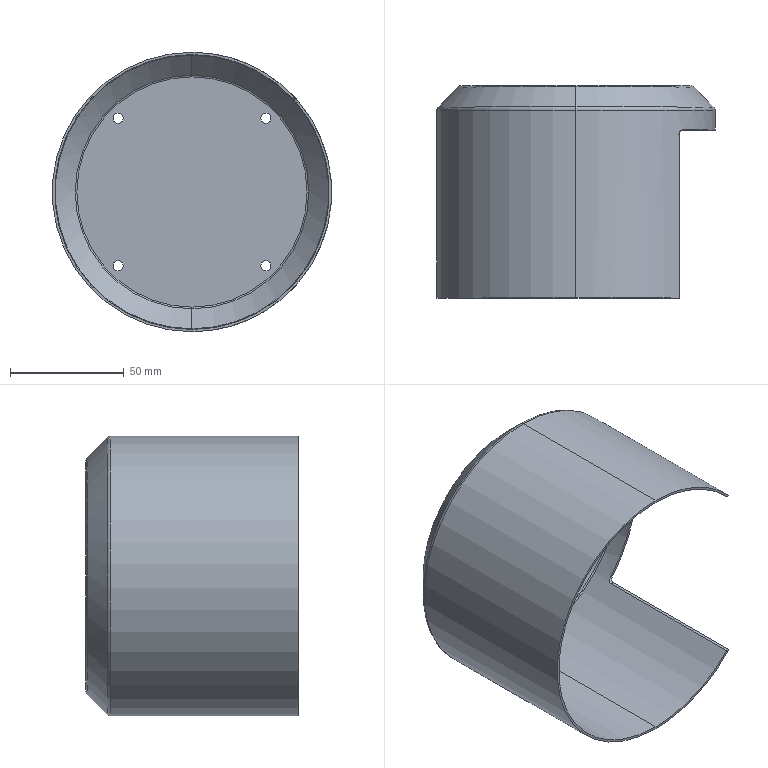Part | SolidWorks | features Fillet 2, Chamfer 1, Extrusion 1, HoleWzd 1, ICE 1, Shell 1 | 1 solid | 32 faces | box 123 x 93.5 x 123 mm | volume 38171 mm3 | cylinder 14 | torus 8 | plane 6 | cone 4 | commonest cylinder face diameters 4.5 x8 4 x2 121 x2 123 x2
STEP:
#1=CARTESIAN_POINT('',(-32.5,45.75,-34.75));
#2=VERTEX_POINT('',#1);
#3=CARTESIAN_POINT('',(-32.5,45.75,-30.25));
#4=VERTEX_POINT('',#3);
#5=CARTESIAN_POINT('',(-32.5,45.75,-32.5));
#6=DIRECTION('',(0.,1.,0.));
#7=DIRECTION('',(0.,0.,1.));
#8=AXIS2_PLACEMENT_3D('',#5,#6,#7);
#9=CIRCLE('',#8,2.25);
#10=EDGE_CURVE('',#2,#4,#9,.T.);
#11=ORIENTED_EDGE('',*,*,#10,.F.);
#12=CARTESIAN_POINT('',(-32.5,46.75,-34.75));
#13=VERTEX_POINT('',#12);
#14=CARTESIAN_POINT('',(-32.5,46.75,-34.75));
#15=DIRECTION('',(0.,1.,0.));
#16=VECTOR('',#15,1000.);
#17=LINE('',#14,#16);
#18=EDGE_CURVE('',#2,#13,#17,.T.);
#19=ORIENTED_EDGE('',*,*,#18,.T.);
#20=CARTESIAN_POINT('',(-32.5,46.75,-30.25));
#21=VERTEX_POINT('',#20);
#22=CARTESIAN_POINT('',(-32.5,46.75,-32.5));
#23=DIRECTION('',(0.,1.,0.));
#24=DIRECTION('',(0.,0.,1.));
#25=AXIS2_PLACEMENT_3D('',#22,#23,#24);
#26=CIRCLE('',#25,2.25);
#27=EDGE_CURVE('',#13,#21,#26,.T.);
#28=ORIENTED_EDGE('',*,*,#27,.T.);
#29=CARTESIAN_POINT('',(-32.5,46.75,-30.25));
#30=DIRECTION('',(0.,1.,0.));
#31=VECTOR('',#30,1000.);
#32=LINE('',#29,#31);
#33=EDGE_CURVE('',#4,#21,#32,.T.);
#34=ORIENTED_EDGE('',*,*,#33,.F.);
#35=EDGE_LOOP('',(#11,#19,#28,#34));
#36=FACE_OUTER_BOUND('',#35,.T.);
#37=CARTESIAN_POINT('',(-32.5,46.75,-32.5));
#38=DIRECTION('',(0.,1.,0.));
#39=DIRECTION('',(0.,0.,1.));
#40=AXIS2_PLACEMENT_3D('',#37,#38,#39);
#41=CYLINDRICAL_SURFACE('',#40,2.25);
#42=ADVANCED_FACE('',(#36),#41,.F.);
#43=CARTESIAN_POINT('',(32.5,45.75,-34.75));
#44=VERTEX_POINT('',#43);
#45=CARTESIAN_POINT('',(32.5,45.75,-30.25));
#46=VERTEX_POINT('',#45);
#47=CARTESIAN_POINT('',(32.5,45.75,-32.5));
#48=DIRECTION('',(0.,1.,0.));
#49=DIRECTION('',(0.,0.,1.));
#50=AXIS2_PLACEMENT_3D('',#47,#48,#49);
#51=CIRCLE('',#50,2.25);
#52=EDGE_CURVE('',#44,#46,#51,.T.);
#53=ORIENTED_EDGE('',*,*,#52,.F.);
#54=CARTESIAN_POINT('',(32.5,46.75,-34.75));
#55=VERTEX_POINT('',#54);
#56=CARTESIAN_POINT('',(32.5,46.75,-34.75));
#57=DIRECTION('',(0.,1.,0.));
#58=VECTOR('',#57,1000.);
#59=LINE('',#56,#58);
#60=EDGE_CURVE('',#44,#55,#59,.T.);
#61=ORIENTED_EDGE('',*,*,#60,.T.);
#62=CARTESIAN_POINT('',(32.5,46.75,-30.25));
#63=VERTEX_POINT('',#62);
#64=CARTESIAN_POINT('',(32.5,46.75,-32.5));
#65=DIRECTION('',(0.,1.,0.));
#66=DIRECTION('',(0.,0.,1.));
#67=AXIS2_PLACEMENT_3D('',#64,#65,#66);
#68=CIRCLE('',#67,2.25);
#69=EDGE_CURVE('',#55,#63,#68,.T.);
#70=ORIENTED_EDGE('',*,*,#69,.T.);
#71=CARTESIAN_POINT('',(32.5,46.75,-30.25));
#72=DIRECTION('',(0.,1.,0.));
#73=VECTOR('',#72,1000.);
#74=LINE('',#71,#73);
#75=EDGE_CURVE('',#46,#63,#74,.T.);
#76=ORIENTED_EDGE('',*,*,#75,.F.);
#77=EDGE_LOOP('',(#53,#61,#70,#76));
#78=FACE_OUTER_BOUND('',#77,.T.);
#79=CARTESIAN_POINT('',(32.5,46.75,-32.5));
#80=DIRECTION('',(0.,1.,0.));
#81=DIRECTION('',(0.,0.,1.));
#82=AXIS2_PLACEMENT_3D('',#79,#80,#81);
#83=CYLINDRICAL_SURFACE('',#82,2.25);
#84=ADVANCED_FACE('',(#78),#83,.F.);
#85=CARTESIAN_POINT('',(32.5,45.75,30.25));
#86=VERTEX_POINT('',#85);
#87=CARTESIAN_POINT('',(32.5,45.75,34.75));
#88=VERTEX_POINT('',#87);
#89=CARTESIAN_POINT('',(32.5,45.75,32.5));
#90=DIRECTION('',(0.,1.,0.));
#91=DIRECTION('',(0.,0.,1.));
#92=AXIS2_PLACEMENT_3D('',#89,#90,#91);
#93=CIRCLE('',#92,2.25);
#94=EDGE_CURVE('',#86,#88,#93,.T.);
#95=ORIENTED_EDGE('',*,*,#94,.F.);
#96=CARTESIAN_POINT('',(32.5,46.75,30.25));
#97=VERTEX_POINT('',#96);
#98=CARTESIAN_POINT('',(32.5,46.75,30.25));
#99=DIRECTION('',(0.,1.,0.));
#100=VECTOR('',#99,1000.);
#101=LINE('',#98,#100);
#102=EDGE_CURVE('',#86,#97,#101,.T.);
#103=ORIENTED_EDGE('',*,*,#102,.T.);
#104=CARTESIAN_POINT('',(32.5,46.75,34.75));
#105=VERTEX_POINT('',#104);
#106=CARTESIAN_POINT('',(32.5,46.75,32.5));
#107=DIRECTION('',(0.,1.,0.));
#108=DIRECTION('',(0.,0.,1.));
#109=AXIS2_PLACEMENT_3D('',#106,#107,#108);
#110=CIRCLE('',#109,2.25);
#111=EDGE_CURVE('',#97,#105,#110,.T.);
#112=ORIENTED_EDGE('',*,*,#111,.T.);
#113=CARTESIAN_POINT('',(32.5,46.75,34.75));
#114=DIRECTION('',(0.,1.,0.));
#115=VECTOR('',#114,1000.);
#116=LINE('',#113,#115);
#117=EDGE_CURVE('',#88,#105,#116,.T.);
#118=ORIENTED_EDGE('',*,*,#117,.F.);
#119=EDGE_LOOP('',(#95,#103,#112,#118));
#120=FACE_OUTER_BOUND('',#119,.T.);
#121=CARTESIAN_POINT('',(32.5,46.75,32.5));
#122=DIRECTION('',(0.,1.,0.));
#123=DIRECTION('',(0.,0.,1.));
#124=AXIS2_PLACEMENT_3D('',#121,#122,#123);
#125=CYLINDRICAL_SURFACE('',#124,2.25);
#126=ADVANCED_FACE('',(#120),#125,.F.);
#127=CARTESIAN_POINT('',(-32.5,45.75,30.25));
#128=VERTEX_POINT('',#127);
#129=CARTESIAN_POINT('',(-32.5,45.75,34.75));
#130=VERTEX_POINT('',#129);
#131=CARTESIAN_POINT('',(-32.5,45.75,32.5));
#132=DIRECTION('',(0.,1.,0.));
#133=DIRECTION('',(0.,0.,1.));
#134=AXIS2_PLACEMENT_3D('',#131,#132,#133);
#135=CIRCLE('',#134,2.25);
#136=EDGE_CURVE('',#128,#130,#135,.T.);
#137=ORIENTED_EDGE('',*,*,#136,.F.);
#138=CARTESIAN_POINT('',(-32.5,46.75,30.25));
#139=VERTEX_POINT('',#138);
#140=CARTESIAN_POINT('',(-32.5,46.75,30.25));
#141=DIRECTION('',(0.,1.,0.));
#142=VECTOR('',#141,1000.);
#143=LINE('',#140,#142);
#144=EDGE_CURVE('',#128,#139,#143,.T.);
#145=ORIENTED_EDGE('',*,*,#144,.T.);
#146=CARTESIAN_POINT('',(-32.5,46.75,34.75));
#147=VERTEX_POINT('',#146);
#148=CARTESIAN_POINT('',(-32.5,46.75,32.5));
#149=DIRECTION('',(0.,1.,0.));
#150=DIRECTION('',(0.,0.,1.));
#151=AXIS2_PLACEMENT_3D('',#148,#149,#150);
#152=CIRCLE('',#151,2.25);
#153=EDGE_CURVE('',#139,#147,#152,.T.);
#154=ORIENTED_EDGE('',*,*,#153,.T.);
#155=CARTESIAN_POINT('',(-32.5,46.75,34.75));
#156=DIRECTION('',(0.,1.,0.));
#157=VECTOR('',#156,1000.);
#158=LINE('',#155,#157);
#159=EDGE_CURVE('',#130,#147,#158,.T.);
#160=ORIENTED_EDGE('',*,*,#159,.F.);
#161=EDGE_LOOP('',(#137,#145,#154,#160));
#162=FACE_OUTER_BOUND('',#161,.T.);
#163=CARTESIAN_POINT('',(-32.5,46.75,32.5));
#164=DIRECTION('',(0.,1.,0.));
#165=DIRECTION('',(0.,0.,1.));
#166=AXIS2_PLACEMENT_3D('',#163,#164,#165);
#167=CYLINDRICAL_SURFACE('',#166,2.25);
#168=ADVANCED_FACE('',(#162),#167,.F.);
#169=CARTESIAN_POINT('',(0.,45.457,51.379));
#170=VERTEX_POINT('',#169);
#171=CARTESIAN_POINT('',(0.,45.457,-51.379));
#172=VERTEX_POINT('',#171);
#173=CARTESIAN_POINT('',(0.,45.457,0.));
#174=DIRECTION('',(0.,-1.,0.));
#175=DIRECTION('',(0.,0.,-1.));
#176=AXIS2_PLACEMENT_3D('',#173,#174,#175);
#177=CIRCLE('',#176,51.379);
#178=EDGE_CURVE('',#170,#172,#177,.T.);
#179=ORIENTED_EDGE('',*,*,#178,.T.);
#180=CARTESIAN_POINT('',(0.,45.75,-50.672));
#181=VERTEX_POINT('',#180);
#182=CARTESIAN_POINT('',(0.,44.75,-50.672));
#183=DIRECTION('',(1.,0.,0.));
#184=DIRECTION('',(0.,0.,-1.));
#185=AXIS2_PLACEMENT_3D('',#182,#183,#184);
#186=CIRCLE('',#185,1.);
#187=EDGE_CURVE('',#172,#181,#186,.T.);
#188=ORIENTED_EDGE('',*,*,#187,.T.);
#189=CARTESIAN_POINT('',(0.,45.75,50.672));
#190=VERTEX_POINT('',#189);
#191=CARTESIAN_POINT('',(0.,45.75,0.));
#192=DIRECTION('',(0.,1.,0.));
#193=DIRECTION('',(0.,0.,1.));
#194=AXIS2_PLACEMENT_3D('',#191,#192,#193);
#195=CIRCLE('',#194,50.672);
#196=EDGE_CURVE('',#181,#190,#195,.T.);
#197=ORIENTED_EDGE('',*,*,#196,.T.);
#198=CARTESIAN_POINT('',(0.,44.75,50.672));
#199=DIRECTION('',(-1.,0.,0.));
#200=DIRECTION('',(0.,0.,1.));
#201=AXIS2_PLACEMENT_3D('',#198,#199,#200);
#202=CIRCLE('',#201,1.);
#203=EDGE_CURVE('',#170,#190,#202,.T.);
#204=ORIENTED_EDGE('',*,*,#203,.F.);
#205=EDGE_LOOP('',(#179,#188,#197,#204));
#206=FACE_OUTER_BOUND('',#205,.T.);
#207=CARTESIAN_POINT('',(0.,44.75,0.));
#208=DIRECTION('',(0.,1.,0.));
#209=DIRECTION('',(0.,0.,1.));
#210=AXIS2_PLACEMENT_3D('',#207,#208,#209);
#211=TOROIDAL_SURFACE('',#210,50.672,1.);
#212=ADVANCED_FACE('',(#206),#211,.F.);
#213=CARTESIAN_POINT('',(0.,35.922,60.5));
#214=VERTEX_POINT('',#213);
#215=CARTESIAN_POINT('',(0.,35.922,-60.5));
#216=VERTEX_POINT('',#215);
#217=CARTESIAN_POINT('',(0.,35.922,0.));
#218=DIRECTION('',(0.,-1.,0.));
#219=DIRECTION('',(0.,0.,-1.));
#220=AXIS2_PLACEMENT_3D('',#217,#218,#219);
#221=CIRCLE('',#220,60.5);
#222=EDGE_CURVE('',#214,#216,#221,.T.);
#223=ORIENTED_EDGE('',*,*,#222,.T.);
#224=CARTESIAN_POINT('',(0.,36.629,-60.207));
#225=VERTEX_POINT('',#224);
#226=CARTESIAN_POINT('',(0.,35.922,-59.5));
#227=DIRECTION('',(1.,0.,0.));
#228=DIRECTION('',(0.,0.,-1.));
#229=AXIS2_PLACEMENT_3D('',#226,#227,#228);
#230=CIRCLE('',#229,1.);
#231=EDGE_CURVE('',#216,#225,#230,.T.);
#232=ORIENTED_EDGE('',*,*,#231,.T.);
#233=CARTESIAN_POINT('',(0.,36.629,60.207));
#234=VERTEX_POINT('',#233);
#235=CARTESIAN_POINT('',(0.,36.629,0.));
#236=DIRECTION('',(0.,1.,0.));
#237=DIRECTION('',(0.,0.,-1.));
#238=AXIS2_PLACEMENT_3D('',#235,#236,#237);
#239=CIRCLE('',#238,60.207);
#240=EDGE_CURVE('',#225,#234,#239,.T.);
#241=ORIENTED_EDGE('',*,*,#240,.T.);
#242=CARTESIAN_POINT('',(0.,35.922,59.5));
#243=DIRECTION('',(-1.,0.,0.));
#244=DIRECTION('',(0.,0.,1.));
#245=AXIS2_PLACEMENT_3D('',#242,#243,#244);
#246=CIRCLE('',#245,1.);
#247=EDGE_CURVE('',#214,#234,#246,.T.);
#248=ORIENTED_EDGE('',*,*,#247,.F.);
#249=EDGE_LOOP('',(#223,#232,#241,#248));
#250=FACE_OUTER_BOUND('',#249,.T.);
#251=CARTESIAN_POINT('',(0.,35.922,0.));
#252=DIRECTION('',(0.,1.,0.));
#253=DIRECTION('',(0.,0.,1.));
#254=AXIS2_PLACEMENT_3D('',#251,#252,#253);
#255=TOROIDAL_SURFACE('',#254,59.5,1.);
#256=ADVANCED_FACE('',(#250),#255,.F.);
#257=ORIENTED_EDGE('',*,*,#178,.F.);
#258=CARTESIAN_POINT('',(0.,46.043,50.793));
#259=DIRECTION('',(0.,-0.7071,0.7071));
#260=VECTOR('',#259,1000.);
#261=LINE('',#258,#260);
#262=EDGE_CURVE('',#170,#234,#261,.T.);
#263=ORIENTED_EDGE('',*,*,#262,.T.);
#264=ORIENTED_EDGE('',*,*,#240,.F.);
#265=CARTESIAN_POINT('',(0.,46.043,-50.793));
#266=DIRECTION('',(0.,-0.7071,-0.7071));
#267=VECTOR('',#266,1000.);
#268=LINE('',#265,#267);
#269=EDGE_CURVE('',#172,#225,#268,.T.);
#270=ORIENTED_EDGE('',*,*,#269,.F.);
#271=EDGE_LOOP('',(#257,#263,#264,#270));
#272=FACE_OUTER_BOUND('',#271,.T.);
#273=CARTESIAN_POINT('',(0.,46.043,0.));
#274=DIRECTION('',(0.,-1.,0.));
#275=DIRECTION('',(0.,0.,-1.));
#276=AXIS2_PLACEMENT_3D('',#273,#274,#275);
#277=CONICAL_SURFACE('',#276,50.793,0.7854);
#278=ADVANCED_FACE('',(#272),#277,.F.);
#279=ORIENTED_EDGE('',*,*,#222,.F.);
#280=CARTESIAN_POINT('',(0.,-46.75,60.5));
#281=VERTEX_POINT('',#280);
#282=CARTESIAN_POINT('',(0.,46.75,60.5));
#283=DIRECTION('',(0.,-1.,0.));
#284=VECTOR('',#283,1000.);
#285=LINE('',#282,#284);
#286=EDGE_CURVE('',#214,#281,#285,.T.);
#287=ORIENTED_EDGE('',*,*,#286,.T.);
#288=CARTESIAN_POINT('',(0.,-46.75,-60.5));
#289=VERTEX_POINT('',#288);
#290=CARTESIAN_POINT('',(0.,-46.75,0.));
#291=DIRECTION('',(0.,1.,0.));
#292=DIRECTION('',(0.,0.,1.));
#293=AXIS2_PLACEMENT_3D('',#290,#291,#292);
#294=CIRCLE('',#293,60.5);
#295=EDGE_CURVE('',#289,#281,#294,.T.);
#296=ORIENTED_EDGE('',*,*,#295,.F.);
#297=CARTESIAN_POINT('',(0.,46.75,-60.5));
#298=DIRECTION('',(0.,-1.,0.));
#299=VECTOR('',#298,1000.);
#300=LINE('',#297,#299);
#301=EDGE_CURVE('',#216,#289,#300,.T.);
#302=ORIENTED_EDGE('',*,*,#301,.F.);
#303=EDGE_LOOP('',(#279,#287,#296,#302));
#304=FACE_OUTER_BOUND('',#303,.T.);
#305=CARTESIAN_POINT('',(0.,46.75,0.));
#306=DIRECTION('',(0.,-1.,0.));
#307=DIRECTION('',(0.,0.,-1.));
#308=AXIS2_PLACEMENT_3D('',#305,#306,#307);
#309=CYLINDRICAL_SURFACE('',#308,60.5);
#310=ADVANCED_FACE('',(#304),#309,.F.);
#311=CARTESIAN_POINT('',(0.,46.164,-52.086));
#312=VERTEX_POINT('',#311);
#313=CARTESIAN_POINT('',(0.,46.164,52.086));
#314=VERTEX_POINT('',#313);
#315=CARTESIAN_POINT('',(0.,46.164,0.));
#316=DIRECTION('',(0.,-1.,0.));
#317=DIRECTION('',(0.,0.,1.));
#318=AXIS2_PLACEMENT_3D('',#315,#316,#317);
#319=CIRCLE('',#318,52.086);
#320=EDGE_CURVE('',#312,#314,#319,.T.);
#321=ORIENTED_EDGE('',*,*,#320,.F.);
#322=CARTESIAN_POINT('',(0.,46.75,-50.672));
#323=VERTEX_POINT('',#322);
#324=CARTESIAN_POINT('',(0.,44.75,-50.672));
#325=DIRECTION('',(1.,0.,0.));
#326=DIRECTION('',(0.,0.,-1.));
#327=AXIS2_PLACEMENT_3D('',#324,#325,#326);
#328=CIRCLE('',#327,2.);
#329=EDGE_CURVE('',#312,#323,#328,.T.);
#330=ORIENTED_EDGE('',*,*,#329,.T.);
#331=CARTESIAN_POINT('',(0.,46.75,50.672));
#332=VERTEX_POINT('',#331);
#333=CARTESIAN_POINT('',(0.,46.75,0.));
#334=DIRECTION('',(0.,1.,0.));
#335=DIRECTION('',(0.,0.,1.));
#336=AXIS2_PLACEMENT_3D('',#333,#334,#335);
#337=CIRCLE('',#336,50.672);
#338=EDGE_CURVE('',#332,#323,#337,.T.);
#339=ORIENTED_EDGE('',*,*,#338,.F.);
#340=CARTESIAN_POINT('',(0.,44.75,50.672));
#341=DIRECTION('',(-1.,0.,0.));
#342=DIRECTION('',(0.,0.,1.));
#343=AXIS2_PLACEMENT_3D('',#340,#341,#342);
#344=CIRCLE('',#343,2.);
#345=EDGE_CURVE('',#314,#332,#344,.T.);
#346=ORIENTED_EDGE('',*,*,#345,.F.);
#347=EDGE_LOOP('',(#321,#330,#339,#346));
#348=FACE_OUTER_BOUND('',#347,.T.);
#349=CARTESIAN_POINT('',(0.,44.75,0.));
#350=DIRECTION('',(0.,1.,0.));
#351=DIRECTION('',(0.,0.,1.));
#352=AXIS2_PLACEMENT_3D('',#349,#350,#351);
#353=TOROIDAL_SURFACE('',#352,50.672,2.);
#354=ADVANCED_FACE('',(#348),#353,.T.);
#355=CARTESIAN_POINT('',(0.,35.922,-61.5));
#356=VERTEX_POINT('',#355);
#357=CARTESIAN_POINT('',(0.,35.922,61.5));
#358=VERTEX_POINT('',#357);
#359=CARTESIAN_POINT('',(0.,35.922,0.));
#360=DIRECTION('',(0.,-1.,0.));
#361=DIRECTION('',(0.,0.,1.));
#362=AXIS2_PLACEMENT_3D('',#359,#360,#361);
#363=CIRCLE('',#362,61.5);
#364=EDGE_CURVE('',#356,#358,#363,.T.);
#365=ORIENTED_EDGE('',*,*,#364,.F.);
#366=CARTESIAN_POINT('',(0.,37.336,-60.914));
#367=VERTEX_POINT('',#366);
#368=CARTESIAN_POINT('',(0.,35.922,-59.5));
#369=DIRECTION('',(1.,0.,0.));
#370=DIRECTION('',(0.,0.,-1.));
#371=AXIS2_PLACEMENT_3D('',#368,#369,#370);
#372=CIRCLE('',#371,2.);
#373=EDGE_CURVE('',#356,#367,#372,.T.);
#374=ORIENTED_EDGE('',*,*,#373,.T.);
#375=CARTESIAN_POINT('',(0.,37.336,60.914));
#376=VERTEX_POINT('',#375);
#377=CARTESIAN_POINT('',(0.,37.336,0.));
#378=DIRECTION('',(0.,1.,0.));
#379=DIRECTION('',(0.,0.,-1.));
#380=AXIS2_PLACEMENT_3D('',#377,#378,#379);
#381=CIRCLE('',#380,60.914);
#382=EDGE_CURVE('',#376,#367,#381,.T.);
#383=ORIENTED_EDGE('',*,*,#382,.F.);
#384=CARTESIAN_POINT('',(0.,35.922,59.5));
#385=DIRECTION('',(-1.,0.,0.));
#386=DIRECTION('',(0.,0.,1.));
#387=AXIS2_PLACEMENT_3D('',#384,#385,#386);
#388=CIRCLE('',#387,2.);
#389=EDGE_CURVE('',#358,#376,#388,.T.);
#390=ORIENTED_EDGE('',*,*,#389,.F.);
#391=EDGE_LOOP('',(#365,#374,#383,#390));
#392=FACE_OUTER_BOUND('',#391,.T.);
#393=CARTESIAN_POINT('',(0.,35.922,0.));
#394=DIRECTION('',(0.,1.,0.));
#395=DIRECTION('',(0.,0.,1.));
#396=AXIS2_PLACEMENT_3D('',#393,#394,#395);
#397=TOROIDAL_SURFACE('',#396,59.5,2.);
#398=ADVANCED_FACE('',(#392),#397,.T.);
#399=ORIENTED_EDGE('',*,*,#320,.T.);
#400=CARTESIAN_POINT('',(0.,46.75,51.5));
#401=DIRECTION('',(0.,-0.7071,0.7071));
#402=VECTOR('',#401,1000.);
#403=LINE('',#400,#402);
#404=EDGE_CURVE('',#314,#376,#403,.T.);
#405=ORIENTED_EDGE('',*,*,#404,.T.);
#406=ORIENTED_EDGE('',*,*,#382,.T.);
#407=CARTESIAN_POINT('',(0.,46.75,-51.5));
#408=DIRECTION('',(0.,-0.7071,-0.7071));
#409=VECTOR('',#408,1000.);
#410=LINE('',#407,#409);
#411=EDGE_CURVE('',#312,#367,#410,.T.);
#412=ORIENTED_EDGE('',*,*,#411,.F.);
#413=EDGE_LOOP('',(#399,#405,#406,#412));
#414=FACE_OUTER_BOUND('',#413,.T.);
#415=CARTESIAN_POINT('',(0.,46.75,0.));
#416=DIRECTION('',(0.,-1.,0.));
#417=DIRECTION('',(0.,0.,-1.));
#418=AXIS2_PLACEMENT_3D('',#415,#416,#417);
#419=CONICAL_SURFACE('',#418,51.5,0.7854);
#420=ADVANCED_FACE('',(#414),#419,.T.);
#421=ORIENTED_EDGE('',*,*,#364,.T.);
#422=CARTESIAN_POINT('',(0.,-46.75,61.5));
#423=VERTEX_POINT('',#422);
#424=CARTESIAN_POINT('',(0.,46.75,61.5));
#425=DIRECTION('',(0.,-1.,0.));
#426=VECTOR('',#425,1000.);
#427=LINE('',#424,#426);
#428=EDGE_CURVE('',#358,#423,#427,.T.);
#429=ORIENTED_EDGE('',*,*,#428,.T.);
#430=CARTESIAN_POINT('',(45.387,-46.75,41.5));
#431=VERTEX_POINT('',#430);
#432=CARTESIAN_POINT('',(0.,-46.75,0.));
#433=DIRECTION('',(0.,1.,0.));
#434=DIRECTION('',(0.,0.,1.));
#435=AXIS2_PLACEMENT_3D('',#432,#433,#434);
#436=CIRCLE('',#435,61.5);
#437=EDGE_CURVE('',#423,#431,#436,.T.);
#438=ORIENTED_EDGE('',*,*,#437,.T.);
#439=CARTESIAN_POINT('',(45.387,25.25,41.5));
#440=VERTEX_POINT('',#439);
#441=CARTESIAN_POINT('',(45.387,46.75,41.5));
#442=DIRECTION('',(0.,1.,0.));
#443=VECTOR('',#442,1000.);
#444=LINE('',#441,#443);
#445=EDGE_CURVE('',#431,#440,#444,.T.);
#446=ORIENTED_EDGE('',*,*,#445,.T.);
#447=CARTESIAN_POINT('',(47.138,27.25,39.5));
#448=VERTEX_POINT('',#447);
#449=CARTESIAN_POINT('',(45.387,25.25,41.5));
#450=CARTESIAN_POINT('',(45.387,25.405,41.5));
#451=CARTESIAN_POINT('',(45.403,25.555,41.482));
#452=CARTESIAN_POINT('',(45.465,25.848,41.414));
#453=CARTESIAN_POINT('',(45.511,25.988,41.364));
#454=CARTESIAN_POINT('',(45.623,26.245,41.241));
#455=CARTESIAN_POINT('',(45.69,26.364,41.166));
#456=CARTESIAN_POINT('',(45.837,26.576,41.003));
#457=CARTESIAN_POINT('',(45.916,26.67,40.914));
#458=CARTESIAN_POINT('',(46.173,26.923,40.625));
#459=CARTESIAN_POINT('',(46.357,27.044,40.415));
#460=CARTESIAN_POINT('',(46.743,27.209,39.968));
#461=CARTESIAN_POINT('',(46.941,27.25,39.736));
#462=CARTESIAN_POINT('',(47.138,27.25,39.5));
#463=B_SPLINE_CURVE_WITH_KNOTS('',3,(#449,#450,#451,#452,#453,#454,#455,#456,#457,#458,#459,#460,#461,#462),.UNSPECIFIED.,.F.,.F.,(4,2,2,2,2,2,4),(0.,0.0004571,0.0009142,0.001371,0.001828,0.002743,0.003657),.UNSPECIFIED.);
#464=EDGE_CURVE('',#440,#448,#463,.T.);
#465=ORIENTED_EDGE('',*,*,#464,.T.);
#466=CARTESIAN_POINT('',(47.138,27.25,-39.5));
#467=VERTEX_POINT('',#466);
#468=CARTESIAN_POINT('',(0.,27.25,0.));
#469=DIRECTION('',(0.,-1.,0.));
#470=DIRECTION('',(0.,0.,-1.));
#471=AXIS2_PLACEMENT_3D('',#468,#469,#470);
#472=CIRCLE('',#471,61.5);
#473=EDGE_CURVE('',#467,#448,#472,.T.);
#474=ORIENTED_EDGE('',*,*,#473,.F.);
#475=CARTESIAN_POINT('',(45.387,25.25,-41.5));
#476=VERTEX_POINT('',#475);
#477=CARTESIAN_POINT('',(47.138,27.25,-39.5));
#478=CARTESIAN_POINT('',(46.94,27.25,-39.736));
#479=CARTESIAN_POINT('',(46.745,27.21,-39.965));
#480=CARTESIAN_POINT('',(46.359,27.046,-40.413));
#481=CARTESIAN_POINT('',(46.173,26.924,-40.624));
#482=CARTESIAN_POINT('',(45.833,26.589,-41.008));
#483=CARTESIAN_POINT('',(45.68,26.375,-41.178));
#484=CARTESIAN_POINT('',(45.511,25.989,-41.364));
#485=CARTESIAN_POINT('',(45.466,25.852,-41.413));
#486=CARTESIAN_POINT('',(45.404,25.557,-41.482));
#487=CARTESIAN_POINT('',(45.387,25.405,-41.5));
#488=CARTESIAN_POINT('',(45.387,25.25,-41.5));
#489=B_SPLINE_CURVE_WITH_KNOTS('',3,(#477,#478,#479,#480,#481,#482,#483,#484,#485,#486,#487,#488),.UNSPECIFIED.,.F.,.F.,(4,2,2,2,2,4),(0.,0.0009127,0.001825,0.002738,0.003194,0.003651),.UNSPECIFIED.);
#490=EDGE_CURVE('',#467,#476,#489,.T.);
#491=ORIENTED_EDGE('',*,*,#490,.T.);
#492=CARTESIAN_POINT('',(45.387,-46.75,-41.5));
#493=VERTEX_POINT('',#492);
#494=CARTESIAN_POINT('',(45.387,46.75,-41.5));
#495=DIRECTION('',(0.,-1.,0.));
#496=VECTOR('',#495,1000.);
#497=LINE('',#494,#496);
#498=EDGE_CURVE('',#476,#493,#497,.T.);
#499=ORIENTED_EDGE('',*,*,#498,.T.);
#500=CARTESIAN_POINT('',(0.,-46.75,-61.5));
#501=VERTEX_POINT('',#500);
#502=CARTESIAN_POINT('',(0.,-46.75,0.));
#503=DIRECTION('',(0.,1.,0.));
#504=DIRECTION('',(0.,0.,1.));
#505=AXIS2_PLACEMENT_3D('',#502,#503,#504);
#506=CIRCLE('',#505,61.5);
#507=EDGE_CURVE('',#493,#501,#506,.T.);
#508=ORIENTED_EDGE('',*,*,#507,.T.);
#509=CARTESIAN_POINT('',(0.,46.75,-61.5));
#510=DIRECTION('',(0.,-1.,0.));
#511=VECTOR('',#510,1000.);
#512=LINE('',#509,#511);
#513=EDGE_CURVE('',#356,#501,#512,.T.);
#514=ORIENTED_EDGE('',*,*,#513,.F.);
#515=EDGE_LOOP('',(#421,#429,#438,#446,#465,#474,#491,#499,#508,#514));
#516=FACE_OUTER_BOUND('',#515,.T.);
#517=CARTESIAN_POINT('',(0.,46.75,0.));
#518=DIRECTION('',(0.,-1.,0.));
#519=DIRECTION('',(0.,0.,-1.));
#520=AXIS2_PLACEMENT_3D('',#517,#518,#519);
#521=CYLINDRICAL_SURFACE('',#520,61.5);
#522=ADVANCED_FACE('',(#516),#521,.T.);
#523=ORIENTED_EDGE('',*,*,#428,.F.);
#524=CARTESIAN_POINT('',(0.,35.922,0.));
#525=DIRECTION('',(0.,-1.,0.));
#526=DIRECTION('',(0.,0.,1.));
#527=AXIS2_PLACEMENT_3D('',#524,#525,#526);
#528=CIRCLE('',#527,61.5);
#529=EDGE_CURVE('',#358,#356,#528,.T.);
#530=ORIENTED_EDGE('',*,*,#529,.T.);
#531=ORIENTED_EDGE('',*,*,#513,.T.);
#532=CARTESIAN_POINT('',(0.,-46.75,0.));
#533=DIRECTION('',(0.,1.,0.));
#534=DIRECTION('',(0.,0.,1.));
#535=AXIS2_PLACEMENT_3D('',#532,#533,#534);
#536=CIRCLE('',#535,61.5);
#537=EDGE_CURVE('',#501,#423,#536,.T.);
#538=ORIENTED_EDGE('',*,*,#537,.T.);
#539=EDGE_LOOP('',(#523,#530,#531,#538));
#540=FACE_OUTER_BOUND('',#539,.T.);
#541=CARTESIAN_POINT('',(0.,46.75,0.));
#542=DIRECTION('',(0.,-1.,0.));
#543=DIRECTION('',(0.,0.,-1.));
#544=AXIS2_PLACEMENT_3D('',#541,#542,#543);
#545=CYLINDRICAL_SURFACE('',#544,61.5);
#546=ADVANCED_FACE('',(#540),#545,.T.);
#547=CARTESIAN_POINT('',(-32.5,46.75,-32.5));
#548=DIRECTION('',(0.,1.,0.));
#549=DIRECTION('',(0.,0.,1.));
#550=AXIS2_PLACEMENT_3D('',#547,#548,#549);
#551=CIRCLE('',#550,2.25);
#552=EDGE_CURVE('',#21,#13,#551,.T.);
#553=ORIENTED_EDGE('',*,*,#552,.F.);
#554=ORIENTED_EDGE('',*,*,#27,.F.);
#555=EDGE_LOOP('',(#553,#554));
#556=FACE_BOUND('',#555,.T.);
#557=CARTESIAN_POINT('',(32.5,46.75,-32.5));
#558=DIRECTION('',(0.,1.,0.));
#559=DIRECTION('',(0.,0.,1.));
#560=AXIS2_PLACEMENT_3D('',#557,#558,#559);
#561=CIRCLE('',#560,2.25);
#562=EDGE_CURVE('',#63,#55,#561,.T.);
#563=ORIENTED_EDGE('',*,*,#562,.F.);
#564=ORIENTED_EDGE('',*,*,#69,.F.);
#565=EDGE_LOOP('',(#563,#564));
#566=FACE_BOUND('',#565,.T.);
#567=CARTESIAN_POINT('',(32.5,46.75,32.5));
#568=DIRECTION('',(0.,1.,0.));
#569=DIRECTION('',(0.,0.,1.));
#570=AXIS2_PLACEMENT_3D('',#567,#568,#569);
#571=CIRCLE('',#570,2.25);
#572=EDGE_CURVE('',#105,#97,#571,.T.);
#573=ORIENTED_EDGE('',*,*,#572,.F.);
#574=ORIENTED_EDGE('',*,*,#111,.F.);
#575=EDGE_LOOP('',(#573,#574));
#576=FACE_BOUND('',#575,.T.);
#577=CARTESIAN_POINT('',(-32.5,46.75,32.5));
#578=DIRECTION('',(0.,1.,0.));
#579=DIRECTION('',(0.,0.,1.));
#580=AXIS2_PLACEMENT_3D('',#577,#578,#579);
#581=CIRCLE('',#580,2.25);
#582=EDGE_CURVE('',#147,#139,#581,.T.);
#583=ORIENTED_EDGE('',*,*,#582,.F.);
#584=ORIENTED_EDGE('',*,*,#153,.F.);
#585=EDGE_LOOP('',(#583,#584));
#586=FACE_BOUND('',#585,.T.);
#587=ORIENTED_EDGE('',*,*,#338,.T.);
#588=CARTESIAN_POINT('',(0.,46.75,0.));
#589=DIRECTION('',(0.,1.,0.));
#590=DIRECTION('',(0.,0.,1.));
#591=AXIS2_PLACEMENT_3D('',#588,#589,#590);
#592=CIRCLE('',#591,50.672);
#593=EDGE_CURVE('',#323,#332,#592,.T.);
#594=ORIENTED_EDGE('',*,*,#593,.T.);
#595=EDGE_LOOP('',(#587,#594));
#596=FACE_OUTER_BOUND('',#595,.T.);
#597=CARTESIAN_POINT('',(0.,46.75,0.));
#598=DIRECTION('',(0.,1.,0.));
#599=DIRECTION('',(0.,0.,1.));
#600=AXIS2_PLACEMENT_3D('',#597,#598,#599);
#601=PLANE('',#600);
#602=ADVANCED_FACE('',(#556,#566,#576,#586,#596),#601,.T.);
#603=ORIENTED_EDGE('',*,*,#507,.F.);
#604=CARTESIAN_POINT('',(44.023,-46.75,-41.5));
#605=VERTEX_POINT('',#604);
#606=CARTESIAN_POINT('',(-5.,-46.75,-41.5));
#607=DIRECTION('',(1.,0.,0.));
#608=VECTOR('',#607,1000.);
#609=LINE('',#606,#608);
#610=EDGE_CURVE('',#605,#493,#609,.T.);
#611=ORIENTED_EDGE('',*,*,#610,.F.);
#612=CARTESIAN_POINT('',(0.,-46.75,0.));
#613=DIRECTION('',(0.,1.,0.));
#614=DIRECTION('',(0.,0.,1.));
#615=AXIS2_PLACEMENT_3D('',#612,#613,#614);
#616=CIRCLE('',#615,60.5);
#617=EDGE_CURVE('',#605,#289,#616,.T.);
#618=ORIENTED_EDGE('',*,*,#617,.T.);
#619=ORIENTED_EDGE('',*,*,#295,.T.);
#620=CARTESIAN_POINT('',(44.023,-46.75,41.5));
#621=VERTEX_POINT('',#620);
#622=CARTESIAN_POINT('',(0.,-46.75,0.));
#623=DIRECTION('',(0.,1.,0.));
#624=DIRECTION('',(0.,0.,1.));
#625=AXIS2_PLACEMENT_3D('',#622,#623,#624);
#626=CIRCLE('',#625,60.5);
#627=EDGE_CURVE('',#281,#621,#626,.T.);
#628=ORIENTED_EDGE('',*,*,#627,.T.);
#629=CARTESIAN_POINT('',(-5.,-46.75,41.5));
#630=DIRECTION('',(-1.,0.,0.));
#631=VECTOR('',#630,1000.);
#632=LINE('',#629,#631);
#633=EDGE_CURVE('',#431,#621,#632,.T.);
#634=ORIENTED_EDGE('',*,*,#633,.F.);
#635=ORIENTED_EDGE('',*,*,#437,.F.);
#636=ORIENTED_EDGE('',*,*,#537,.F.);
#637=EDGE_LOOP('',(#603,#611,#618,#619,#628,#634,#635,#636));
#638=FACE_OUTER_BOUND('',#637,.T.);
#639=CARTESIAN_POINT('',(0.,-46.75,0.));
#640=DIRECTION('',(0.,1.,0.));
#641=DIRECTION('',(0.,0.,1.));
#642=AXIS2_PLACEMENT_3D('',#639,#640,#641);
#643=PLANE('',#642);
#644=ADVANCED_FACE('',(#638),#643,.F.);
#645=ORIENTED_EDGE('',*,*,#404,.F.);
#646=CARTESIAN_POINT('',(0.,46.164,0.));
#647=DIRECTION('',(0.,-1.,0.));
#648=DIRECTION('',(0.,0.,1.));
#649=AXIS2_PLACEMENT_3D('',#646,#647,#648);
#650=CIRCLE('',#649,52.086);
#651=EDGE_CURVE('',#314,#312,#650,.T.);
#652=ORIENTED_EDGE('',*,*,#651,.T.);
#653=ORIENTED_EDGE('',*,*,#411,.T.);
#654=CARTESIAN_POINT('',(0.,37.336,0.));
#655=DIRECTION('',(0.,1.,0.));
#656=DIRECTION('',(0.,0.,-1.));
#657=AXIS2_PLACEMENT_3D('',#654,#655,#656);
#658=CIRCLE('',#657,60.914);
#659=EDGE_CURVE('',#367,#376,#658,.T.);
#660=ORIENTED_EDGE('',*,*,#659,.T.);
#661=EDGE_LOOP('',(#645,#652,#653,#660));
#662=FACE_OUTER_BOUND('',#661,.T.);
#663=CARTESIAN_POINT('',(0.,46.75,0.));
#664=DIRECTION('',(0.,-1.,0.));
#665=DIRECTION('',(0.,0.,-1.));
#666=AXIS2_PLACEMENT_3D('',#663,#664,#665);
#667=CONICAL_SURFACE('',#666,51.5,0.7854);
#668=ADVANCED_FACE('',(#662),#667,.T.);
#669=ORIENTED_EDGE('',*,*,#373,.F.);
#670=ORIENTED_EDGE('',*,*,#529,.F.);
#671=ORIENTED_EDGE('',*,*,#389,.T.);
#672=ORIENTED_EDGE('',*,*,#659,.F.);
#673=EDGE_LOOP('',(#669,#670,#671,#672));
#674=FACE_OUTER_BOUND('',#673,.T.);
#675=CARTESIAN_POINT('',(0.,35.922,0.));
#676=DIRECTION('',(0.,1.,0.));
#677=DIRECTION('',(0.,0.,1.));
#678=AXIS2_PLACEMENT_3D('',#675,#676,#677);
#679=TOROIDAL_SURFACE('',#678,59.5,2.);
#680=ADVANCED_FACE('',(#674),#679,.T.);
#681=ORIENTED_EDGE('',*,*,#329,.F.);
#682=ORIENTED_EDGE('',*,*,#651,.F.);
#683=ORIENTED_EDGE('',*,*,#345,.T.);
#684=ORIENTED_EDGE('',*,*,#593,.F.);
#685=EDGE_LOOP('',(#681,#682,#683,#684));
#686=FACE_OUTER_BOUND('',#685,.T.);
#687=CARTESIAN_POINT('',(0.,44.75,0.));
#688=DIRECTION('',(0.,1.,0.));
#689=DIRECTION('',(0.,0.,1.));
#690=AXIS2_PLACEMENT_3D('',#687,#688,#689);
#691=TOROIDAL_SURFACE('',#690,50.672,2.);
#692=ADVANCED_FACE('',(#686),#691,.T.);
#693=ORIENTED_EDGE('',*,*,#286,.F.);
#694=CARTESIAN_POINT('',(0.,35.922,0.));
#695=DIRECTION('',(0.,-1.,0.));
#696=DIRECTION('',(0.,0.,-1.));
#697=AXIS2_PLACEMENT_3D('',#694,#695,#696);
#698=CIRCLE('',#697,60.5);
#699=EDGE_CURVE('',#216,#214,#698,.T.);
#700=ORIENTED_EDGE('',*,*,#699,.F.);
#701=ORIENTED_EDGE('',*,*,#301,.T.);
#702=ORIENTED_EDGE('',*,*,#617,.F.);
#703=CARTESIAN_POINT('',(44.023,25.25,-41.5));
#704=VERTEX_POINT('',#703);
#705=CARTESIAN_POINT('',(44.023,46.75,-41.5));
#706=DIRECTION('',(0.,-1.,0.));
#707=VECTOR('',#706,1000.);
#708=LINE('',#705,#707);
#709=EDGE_CURVE('',#704,#605,#708,.T.);
#710=ORIENTED_EDGE('',*,*,#709,.F.);
#711=CARTESIAN_POINT('',(45.826,27.25,-39.5));
#712=VERTEX_POINT('',#711);
#713=CARTESIAN_POINT('',(44.023,25.25,-41.5));
#714=CARTESIAN_POINT('',(44.023,25.406,-41.5));
#715=CARTESIAN_POINT('',(44.04,25.558,-41.482));
#716=CARTESIAN_POINT('',(44.105,25.853,-41.413));
#717=CARTESIAN_POINT('',(44.152,25.993,-41.362));
#718=CARTESIAN_POINT('',(44.268,26.25,-41.238));
#719=CARTESIAN_POINT('',(44.338,26.369,-41.163));
#720=CARTESIAN_POINT('',(44.49,26.58,-40.999));
#721=CARTESIAN_POINT('',(44.572,26.674,-40.91));
#722=CARTESIAN_POINT('',(44.836,26.926,-40.62));
#723=CARTESIAN_POINT('',(45.025,27.046,-40.411));
#724=CARTESIAN_POINT('',(45.421,27.209,-39.966));
#725=CARTESIAN_POINT('',(45.623,27.25,-39.735));
#726=CARTESIAN_POINT('',(45.826,27.25,-39.5));
#727=B_SPLINE_CURVE_WITH_KNOTS('',3,(#713,#714,#715,#716,#717,#718,#719,#720,#721,#722,#723,#724,#725,#726),.UNSPECIFIED.,.F.,.F.,(4,2,2,2,2,2,4),(0.,0.0004607,0.0009214,0.001382,0.001843,0.002764,0.003686),.UNSPECIFIED.);
#728=EDGE_CURVE('',#704,#712,#727,.T.);
#729=ORIENTED_EDGE('',*,*,#728,.T.);
#730=CARTESIAN_POINT('',(45.826,27.25,39.5));
#731=VERTEX_POINT('',#730);
#732=CARTESIAN_POINT('',(0.,27.25,0.));
#733=DIRECTION('',(0.,-1.,0.));
#734=DIRECTION('',(0.,0.,-1.));
#735=AXIS2_PLACEMENT_3D('',#732,#733,#734);
#736=CIRCLE('',#735,60.5);
#737=EDGE_CURVE('',#712,#731,#736,.T.);
#738=ORIENTED_EDGE('',*,*,#737,.T.);
#739=CARTESIAN_POINT('',(44.023,25.25,41.5));
#740=VERTEX_POINT('',#739);
#741=CARTESIAN_POINT('',(45.826,27.25,39.5));
#742=CARTESIAN_POINT('',(45.623,27.25,39.735));
#743=CARTESIAN_POINT('',(45.423,27.21,39.964));
#744=CARTESIAN_POINT('',(45.027,27.047,40.409));
#745=CARTESIAN_POINT('',(44.837,26.926,40.62));
#746=CARTESIAN_POINT('',(44.486,26.593,41.004));
#747=CARTESIAN_POINT('',(44.328,26.38,41.175));
#748=CARTESIAN_POINT('',(44.152,25.993,41.362));
#749=CARTESIAN_POINT('',(44.105,25.856,41.412));
#750=CARTESIAN_POINT('',(44.04,25.559,41.482));
#751=CARTESIAN_POINT('',(44.023,25.406,41.5));
#752=CARTESIAN_POINT('',(44.023,25.25,41.5));
#753=B_SPLINE_CURVE_WITH_KNOTS('',3,(#741,#742,#743,#744,#745,#746,#747,#748,#749,#750,#751,#752),.UNSPECIFIED.,.F.,.F.,(4,2,2,2,2,4),(0.,0.0009202,0.00184,0.002761,0.003221,0.003681),.UNSPECIFIED.);
#754=EDGE_CURVE('',#731,#740,#753,.T.);
#755=ORIENTED_EDGE('',*,*,#754,.T.);
#756=CARTESIAN_POINT('',(44.023,46.75,41.5));
#757=DIRECTION('',(0.,1.,0.));
#758=VECTOR('',#757,1000.);
#759=LINE('',#756,#758);
#760=EDGE_CURVE('',#621,#740,#759,.T.);
#761=ORIENTED_EDGE('',*,*,#760,.F.);
#762=ORIENTED_EDGE('',*,*,#627,.F.);
#763=EDGE_LOOP('',(#693,#700,#701,#702,#710,#729,#738,#755,#761,#762));
#764=FACE_OUTER_BOUND('',#763,.T.);
#765=CARTESIAN_POINT('',(0.,46.75,0.));
#766=DIRECTION('',(0.,-1.,0.));
#767=DIRECTION('',(0.,0.,-1.));
#768=AXIS2_PLACEMENT_3D('',#765,#766,#767);
#769=CYLINDRICAL_SURFACE('',#768,60.5);
#770=ADVANCED_FACE('',(#764),#769,.F.);
#771=CARTESIAN_POINT('',(-32.5,45.75,-32.5));
#772=DIRECTION('',(0.,1.,0.));
#773=DIRECTION('',(0.,0.,1.));
#774=AXIS2_PLACEMENT_3D('',#771,#772,#773);
#775=CIRCLE('',#774,2.25);
#776=EDGE_CURVE('',#4,#2,#775,.T.);
#777=ORIENTED_EDGE('',*,*,#776,.T.);
#778=ORIENTED_EDGE('',*,*,#10,.T.);
#779=EDGE_LOOP('',(#777,#778));
#780=FACE_BOUND('',#779,.T.);
#781=CARTESIAN_POINT('',(32.5,45.75,-32.5));
#782=DIRECTION('',(0.,1.,0.));
#783=DIRECTION('',(0.,0.,1.));
#784=AXIS2_PLACEMENT_3D('',#781,#782,#783);
#785=CIRCLE('',#784,2.25);
#786=EDGE_CURVE('',#46,#44,#785,.T.);
#787=ORIENTED_EDGE('',*,*,#786,.T.);
#788=ORIENTED_EDGE('',*,*,#52,.T.);
#789=EDGE_LOOP('',(#787,#788));
#790=FACE_BOUND('',#789,.T.);
#791=CARTESIAN_POINT('',(32.5,45.75,32.5));
#792=DIRECTION('',(0.,1.,0.));
#793=DIRECTION('',(0.,0.,1.));
#794=AXIS2_PLACEMENT_3D('',#791,#792,#793);
#795=CIRCLE('',#794,2.25);
#796=EDGE_CURVE('',#88,#86,#795,.T.);
#797=ORIENTED_EDGE('',*,*,#796,.T.);
#798=ORIENTED_EDGE('',*,*,#94,.T.);
#799=EDGE_LOOP('',(#797,#798));
#800=FACE_BOUND('',#799,.T.);
#801=CARTESIAN_POINT('',(-32.5,45.75,32.5));
#802=DIRECTION('',(0.,1.,0.));
#803=DIRECTION('',(0.,0.,1.));
#804=AXIS2_PLACEMENT_3D('',#801,#802,#803);
#805=CIRCLE('',#804,2.25);
#806=EDGE_CURVE('',#130,#128,#805,.T.);
#807=ORIENTED_EDGE('',*,*,#806,.T.);
#808=ORIENTED_EDGE('',*,*,#136,.T.);
#809=EDGE_LOOP('',(#807,#808));
#810=FACE_BOUND('',#809,.T.);
#811=CARTESIAN_POINT('',(0.,45.75,0.));
#812=DIRECTION('',(0.,1.,0.));
#813=DIRECTION('',(0.,0.,1.));
#814=AXIS2_PLACEMENT_3D('',#811,#812,#813);
#815=CIRCLE('',#814,50.672);
#816=EDGE_CURVE('',#190,#181,#815,.T.);
#817=ORIENTED_EDGE('',*,*,#816,.F.);
#818=ORIENTED_EDGE('',*,*,#196,.F.);
#819=EDGE_LOOP('',(#817,#818));
#820=FACE_OUTER_BOUND('',#819,.T.);
#821=CARTESIAN_POINT('',(0.,45.75,0.));
#822=DIRECTION('',(0.,1.,0.));
#823=DIRECTION('',(0.,0.,1.));
#824=AXIS2_PLACEMENT_3D('',#821,#822,#823);
#825=PLANE('',#824);
#826=ADVANCED_FACE('',(#780,#790,#800,#810,#820),#825,.F.);
#827=ORIENTED_EDGE('',*,*,#262,.F.);
#828=CARTESIAN_POINT('',(0.,45.457,0.));
#829=DIRECTION('',(0.,-1.,0.));
#830=DIRECTION('',(0.,0.,-1.));
#831=AXIS2_PLACEMENT_3D('',#828,#829,#830);
#832=CIRCLE('',#831,51.379);
#833=EDGE_CURVE('',#172,#170,#832,.T.);
#834=ORIENTED_EDGE('',*,*,#833,.F.);
#835=ORIENTED_EDGE('',*,*,#269,.T.);
#836=CARTESIAN_POINT('',(0.,36.629,0.));
#837=DIRECTION('',(0.,1.,0.));
#838=DIRECTION('',(0.,0.,-1.));
#839=AXIS2_PLACEMENT_3D('',#836,#837,#838);
#840=CIRCLE('',#839,60.207);
#841=EDGE_CURVE('',#234,#225,#840,.T.);
#842=ORIENTED_EDGE('',*,*,#841,.F.);
#843=EDGE_LOOP('',(#827,#834,#835,#842));
#844=FACE_OUTER_BOUND('',#843,.T.);
#845=CARTESIAN_POINT('',(0.,46.043,0.));
#846=DIRECTION('',(0.,-1.,0.));
#847=DIRECTION('',(0.,0.,-1.));
#848=AXIS2_PLACEMENT_3D('',#845,#846,#847);
#849=CONICAL_SURFACE('',#848,50.793,0.7854);
#850=ADVANCED_FACE('',(#844),#849,.F.);
#851=ORIENTED_EDGE('',*,*,#231,.F.);
#852=ORIENTED_EDGE('',*,*,#699,.T.);
#853=ORIENTED_EDGE('',*,*,#247,.T.);
#854=ORIENTED_EDGE('',*,*,#841,.T.);
#855=EDGE_LOOP('',(#851,#852,#853,#854));
#856=FACE_OUTER_BOUND('',#855,.T.);
#857=CARTESIAN_POINT('',(0.,35.922,0.));
#858=DIRECTION('',(0.,1.,0.));
#859=DIRECTION('',(0.,0.,1.));
#860=AXIS2_PLACEMENT_3D('',#857,#858,#859);
#861=TOROIDAL_SURFACE('',#860,59.5,1.);
#862=ADVANCED_FACE('',(#856),#861,.F.);
#863=ORIENTED_EDGE('',*,*,#187,.F.);
#864=ORIENTED_EDGE('',*,*,#833,.T.);
#865=ORIENTED_EDGE('',*,*,#203,.T.);
#866=ORIENTED_EDGE('',*,*,#816,.T.);
#867=EDGE_LOOP('',(#863,#864,#865,#866));
#868=FACE_OUTER_BOUND('',#867,.T.);
#869=CARTESIAN_POINT('',(0.,44.75,0.));
#870=DIRECTION('',(0.,1.,0.));
#871=DIRECTION('',(0.,0.,1.));
#872=AXIS2_PLACEMENT_3D('',#869,#870,#871);
#873=TOROIDAL_SURFACE('',#872,50.672,1.);
#874=ADVANCED_FACE('',(#868),#873,.F.);
#875=ORIENTED_EDGE('',*,*,#144,.F.);
#876=ORIENTED_EDGE('',*,*,#806,.F.);
#877=ORIENTED_EDGE('',*,*,#159,.T.);
#878=ORIENTED_EDGE('',*,*,#582,.T.);
#879=EDGE_LOOP('',(#875,#876,#877,#878));
#880=FACE_OUTER_BOUND('',#879,.T.);
#881=CARTESIAN_POINT('',(-32.5,46.75,32.5));
#882=DIRECTION('',(0.,1.,0.));
#883=DIRECTION('',(0.,0.,1.));
#884=AXIS2_PLACEMENT_3D('',#881,#882,#883);
#885=CYLINDRICAL_SURFACE('',#884,2.25);
#886=ADVANCED_FACE('',(#880),#885,.F.);
#887=ORIENTED_EDGE('',*,*,#102,.F.);
#888=ORIENTED_EDGE('',*,*,#796,.F.);
#889=ORIENTED_EDGE('',*,*,#117,.T.);
#890=ORIENTED_EDGE('',*,*,#572,.T.);
#891=EDGE_LOOP('',(#887,#888,#889,#890));
#892=FACE_OUTER_BOUND('',#891,.T.);
#893=CARTESIAN_POINT('',(32.5,46.75,32.5));
#894=DIRECTION('',(0.,1.,0.));
#895=DIRECTION('',(0.,0.,1.));
#896=AXIS2_PLACEMENT_3D('',#893,#894,#895);
#897=CYLINDRICAL_SURFACE('',#896,2.25);
#898=ADVANCED_FACE('',(#892),#897,.F.);
#899=ORIENTED_EDGE('',*,*,#60,.F.);
#900=ORIENTED_EDGE('',*,*,#786,.F.);
#901=ORIENTED_EDGE('',*,*,#75,.T.);
#902=ORIENTED_EDGE('',*,*,#562,.T.);
#903=EDGE_LOOP('',(#899,#900,#901,#902));
#904=FACE_OUTER_BOUND('',#903,.T.);
#905=CARTESIAN_POINT('',(32.5,46.75,-32.5));
#906=DIRECTION('',(0.,1.,0.));
#907=DIRECTION('',(0.,0.,1.));
#908=AXIS2_PLACEMENT_3D('',#905,#906,#907);
#909=CYLINDRICAL_SURFACE('',#908,2.25);
#910=ADVANCED_FACE('',(#904),#909,.F.);
#911=ORIENTED_EDGE('',*,*,#18,.F.);
#912=ORIENTED_EDGE('',*,*,#776,.F.);
#913=ORIENTED_EDGE('',*,*,#33,.T.);
#914=ORIENTED_EDGE('',*,*,#552,.T.);
#915=EDGE_LOOP('',(#911,#912,#913,#914));
#916=FACE_OUTER_BOUND('',#915,.T.);
#917=CARTESIAN_POINT('',(-32.5,46.75,-32.5));
#918=DIRECTION('',(0.,1.,0.));
#919=DIRECTION('',(0.,0.,1.));
#920=AXIS2_PLACEMENT_3D('',#917,#918,#919);
#921=CYLINDRICAL_SURFACE('',#920,2.25);
#922=ADVANCED_FACE('',(#916),#921,.F.);
#923=ORIENTED_EDGE('',*,*,#498,.F.);
#924=CARTESIAN_POINT('',(-5.,25.25,-41.5));
#925=DIRECTION('',(-1.,0.,0.));
#926=VECTOR('',#925,1000.);
#927=LINE('',#924,#926);
#928=EDGE_CURVE('',#476,#704,#927,.T.);
#929=ORIENTED_EDGE('',*,*,#928,.T.);
#930=ORIENTED_EDGE('',*,*,#709,.T.);
#931=ORIENTED_EDGE('',*,*,#610,.T.);
#932=EDGE_LOOP('',(#923,#929,#930,#931));
#933=FACE_OUTER_BOUND('',#932,.T.);
#934=CARTESIAN_POINT('',(-5.,27.25,-41.5));
#935=DIRECTION('',(0.,0.,-1.));
#936=DIRECTION('',(-1.,0.,0.));
#937=AXIS2_PLACEMENT_3D('',#934,#935,#936);
#938=PLANE('',#937);
#939=ADVANCED_FACE('',(#933),#938,.F.);
#940=ORIENTED_EDGE('',*,*,#760,.T.);
#941=CARTESIAN_POINT('',(-5.,25.25,41.5));
#942=DIRECTION('',(1.,0.,0.));
#943=VECTOR('',#942,1000.);
#944=LINE('',#941,#943);
#945=EDGE_CURVE('',#740,#440,#944,.T.);
#946=ORIENTED_EDGE('',*,*,#945,.T.);
#947=ORIENTED_EDGE('',*,*,#445,.F.);
#948=ORIENTED_EDGE('',*,*,#633,.T.);
#949=EDGE_LOOP('',(#940,#946,#947,#948));
#950=FACE_OUTER_BOUND('',#949,.T.);
#951=CARTESIAN_POINT('',(-5.,27.25,41.5));
#952=DIRECTION('',(0.,0.,1.));
#953=DIRECTION('',(1.,0.,0.));
#954=AXIS2_PLACEMENT_3D('',#951,#952,#953);
#955=PLANE('',#954);
#956=ADVANCED_FACE('',(#950),#955,.F.);
#957=ORIENTED_EDGE('',*,*,#473,.T.);
#958=CARTESIAN_POINT('',(0.,27.25,39.5));
#959=DIRECTION('',(-1.,0.,0.));
#960=VECTOR('',#959,1000.);
#961=LINE('',#958,#960);
#962=EDGE_CURVE('',#448,#731,#961,.T.);
#963=ORIENTED_EDGE('',*,*,#962,.T.);
#964=ORIENTED_EDGE('',*,*,#737,.F.);
#965=CARTESIAN_POINT('',(0.,27.25,-39.5));
#966=DIRECTION('',(1.,0.,0.));
#967=VECTOR('',#966,1000.);
#968=LINE('',#965,#967);
#969=EDGE_CURVE('',#712,#467,#968,.T.);
#970=ORIENTED_EDGE('',*,*,#969,.T.);
#971=EDGE_LOOP('',(#957,#963,#964,#970));
#972=FACE_OUTER_BOUND('',#971,.T.);
#973=CARTESIAN_POINT('',(0.,27.25,0.));
#974=DIRECTION('',(0.,-1.,0.));
#975=DIRECTION('',(0.,0.,-1.));
#976=AXIS2_PLACEMENT_3D('',#973,#974,#975);
#977=PLANE('',#976);
#978=ADVANCED_FACE('',(#972),#977,.T.);
#979=ORIENTED_EDGE('',*,*,#464,.F.);
#980=ORIENTED_EDGE('',*,*,#945,.F.);
#981=ORIENTED_EDGE('',*,*,#754,.F.);
#982=ORIENTED_EDGE('',*,*,#962,.F.);
#983=EDGE_LOOP('',(#979,#980,#981,#982));
#984=FACE_OUTER_BOUND('',#983,.T.);
#985=CARTESIAN_POINT('',(0.,25.25,39.5));
#986=DIRECTION('',(-1.,0.,0.));
#987=DIRECTION('',(0.,0.,1.));
#988=AXIS2_PLACEMENT_3D('',#985,#986,#987);
#989=CYLINDRICAL_SURFACE('',#988,2.);
#990=ADVANCED_FACE('',(#984),#989,.F.);
#991=ORIENTED_EDGE('',*,*,#728,.F.);
#992=ORIENTED_EDGE('',*,*,#928,.F.);
#993=ORIENTED_EDGE('',*,*,#490,.F.);
#994=ORIENTED_EDGE('',*,*,#969,.F.);
#995=EDGE_LOOP('',(#991,#992,#993,#994));
#996=FACE_OUTER_BOUND('',#995,.T.);
#997=CARTESIAN_POINT('',(0.,25.25,-39.5));
#998=DIRECTION('',(1.,0.,0.));
#999=DIRECTION('',(0.,0.,-1.));
#1000=AXIS2_PLACEMENT_3D('',#997,#998,#999);
#1001=CYLINDRICAL_SURFACE('',#1000,2.);
#1002=ADVANCED_FACE('',(#996),#1001,.F.);
#1003=CLOSED_SHELL('',(#42,#84,#126,#168,#212,#256,#278,#310,#354,#398,#420,#522,#546,#602,#644,#668,#680,#692,#770,#826,#850,#862,#874,#886,#898,#910,#922,#939,#956,#978,#990,#1002));
#1004=MANIFOLD_SOLID_BREP('',#1003);
#1005=CARTESIAN_POINT('',(0.,0.,0.));
#1006=DIRECTION('',(0.,0.,1.));
#1007=DIRECTION('',(1.,0.,0.));
#1008=AXIS2_PLACEMENT_3D('',#1005,#1006,#1007);
#1009=(LENGTH_UNIT()NAMED_UNIT(*)SI_UNIT(.MILLI.,.METRE.));
#1010=UNCERTAINTY_MEASURE_WITH_UNIT(LENGTH_MEASURE(0.00001),#1009,'','');
#1011=(NAMED_UNIT(*)PLANE_ANGLE_UNIT()SI_UNIT($,.RADIAN.));
#1012=(NAMED_UNIT(*)SI_UNIT($,.STERADIAN.)SOLID_ANGLE_UNIT());
#1013=(GEOMETRIC_REPRESENTATION_CONTEXT(3)GLOBAL_UNCERTAINTY_ASSIGNED_CONTEXT((#1010))GLOBAL_UNIT_ASSIGNED_CONTEXT((#1009,#1011,#1012))REPRESENTATION_CONTEXT('',''));
#1014=ADVANCED_BREP_SHAPE_REPRESENTATION('',(#1004,#1008),#1013);